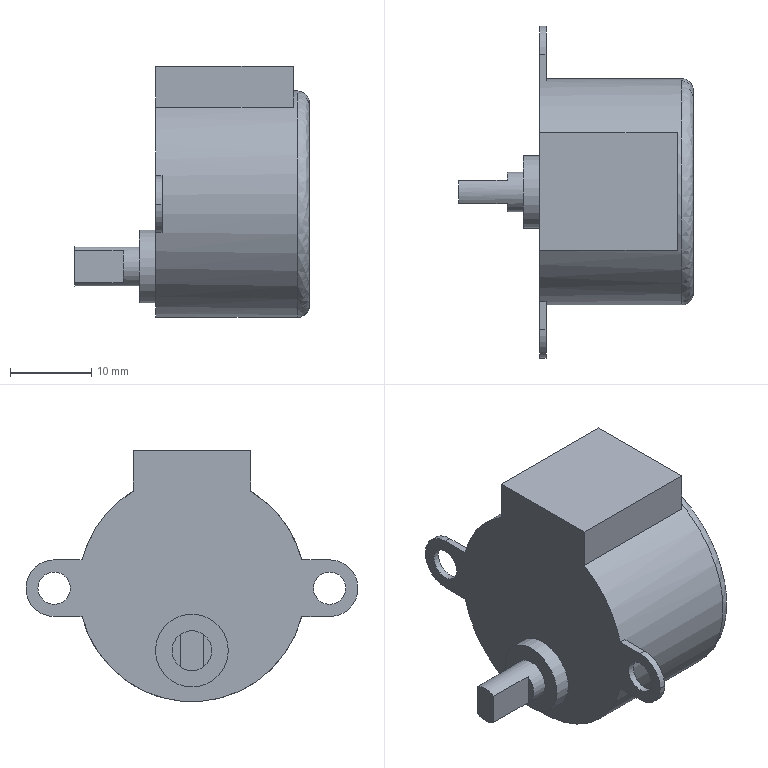Part | STEP file | Wytnij-wyci_gni_cie1_6 | 1 solid | 27 faces | box 29 x 41 x 31 mm | volume 12849 mm3 | plane 18 | cylinder 8 | spline 1 | commonest cylinder face diameters 7 x3 4 x2 4.9 x1 9 x1 28 x1